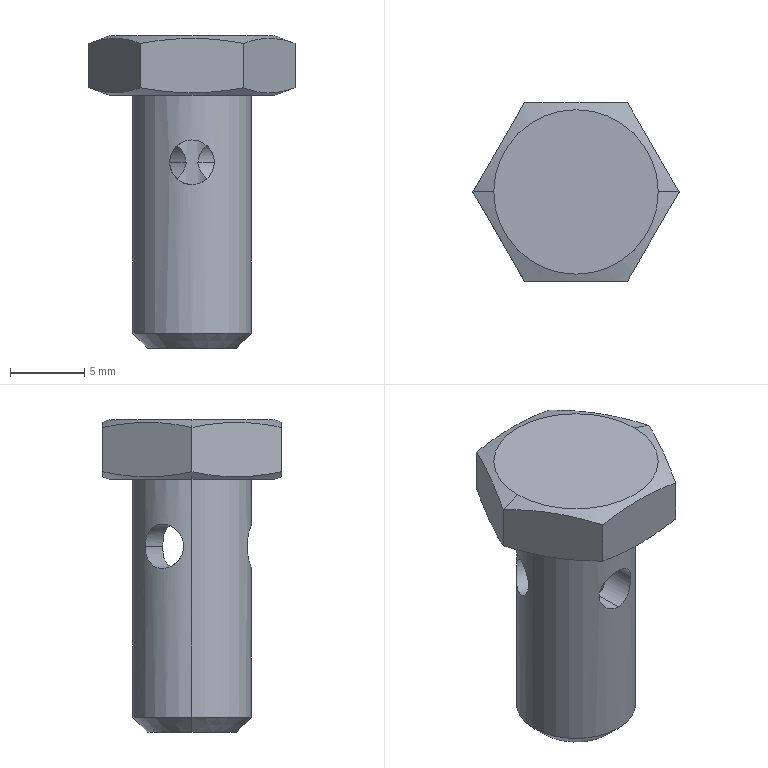Part | SolidWorks | features BaseBody 1 | 1 solid | 26 faces | box 13.856 x 12 x 21 mm | volume 1075 mm3 | cylinder 10 | plane 10 | cone 6 | commonest cylinder face diameters 3 x6 4 x2 8 x2
STEP:
#1=CARTESIAN_POINT('',(-2.461,3.153,-8.5));
#2=VERTEX_POINT('',#1);
#3=CARTESIAN_POINT('',(-3.961,0.555,-8.5));
#4=VERTEX_POINT('',#3);
#5=CARTESIAN_POINT('',(-2.461,3.153,-8.5));
#6=CARTESIAN_POINT('',(-2.461,3.153,-8.4));
#7=CARTESIAN_POINT('',(-2.47,3.147,-8.302));
#8=CARTESIAN_POINT('',(-2.502,3.121,-8.109));
#9=CARTESIAN_POINT('',(-2.527,3.101,-8.013));
#10=CARTESIAN_POINT('',(-2.62,3.024,-7.742));
#11=CARTESIAN_POINT('',(-2.709,2.947,-7.577));
#12=CARTESIAN_POINT('',(-2.911,2.747,-7.303));
#13=CARTESIAN_POINT('',(-3.026,2.623,-7.191));
#14=CARTESIAN_POINT('',(-3.195,2.408,-7.078));
#15=CARTESIAN_POINT('',(-3.252,2.331,-7.049));
#16=CARTESIAN_POINT('',(-3.362,2.17,-7.01));
#17=CARTESIAN_POINT('',(-3.414,2.087,-7.));
#18=CARTESIAN_POINT('',(-3.513,1.916,-7.));
#19=CARTESIAN_POINT('',(-3.56,1.827,-7.01));
#20=CARTESIAN_POINT('',(-3.644,1.653,-7.048));
#21=CARTESIAN_POINT('',(-3.682,1.566,-7.077));
#22=CARTESIAN_POINT('',(-3.784,1.308,-7.191));
#23=CARTESIAN_POINT('',(-3.834,1.148,-7.302));
#24=CARTESIAN_POINT('',(-3.888,0.941,-7.508));
#25=CARTESIAN_POINT('',(-3.903,0.8782,-7.583));
#26=CARTESIAN_POINT('',(-3.926,0.7663,-7.744));
#27=CARTESIAN_POINT('',(-3.935,0.7172,-7.832));
#28=CARTESIAN_POINT('',(-3.956,0.5987,-8.102));
#29=CARTESIAN_POINT('',(-3.961,0.555,-8.3));
#30=CARTESIAN_POINT('',(-3.961,0.555,-8.5));
#31=B_SPLINE_CURVE_WITH_KNOTS('',3,(#5,#6,#7,#8,#9,#10,#11,#12,#13,#14,#15,#16,#17,#18,#19,#20,#21,#22,#23,#24,#25,#26,#27,#28,#29,#30),.UNSPECIFIED.,.F.,.F.,(4,2,2,2,2,2,2,2,2,2,2,2,4),(0.004731,0.005027,0.005322,0.005914,0.006505,0.006801,0.007096,0.007392,0.007688,0.008279,0.008575,0.00887,0.009461),.UNSPECIFIED.);
#32=EDGE_CURVE('',#2,#4,#31,.T.);
#33=ORIENTED_EDGE('',*,*,#32,.T.);
#34=CARTESIAN_POINT('',(-3.961,0.555,-8.5));
#35=CARTESIAN_POINT('',(-3.961,0.555,-8.6));
#36=CARTESIAN_POINT('',(-3.96,0.5656,-8.698));
#37=CARTESIAN_POINT('',(-3.954,0.6067,-8.891));
#38=CARTESIAN_POINT('',(-3.949,0.6378,-8.987));
#39=CARTESIAN_POINT('',(-3.929,0.7568,-9.258));
#40=CARTESIAN_POINT('',(-3.906,0.8722,-9.423));
#41=CARTESIAN_POINT('',(-3.835,1.147,-9.697));
#42=CARTESIAN_POINT('',(-3.784,1.309,-9.809));
#43=CARTESIAN_POINT('',(-3.683,1.563,-9.922));
#44=CARTESIAN_POINT('',(-3.645,1.651,-9.951));
#45=CARTESIAN_POINT('',(-3.56,1.826,-9.99));
#46=CARTESIAN_POINT('',(-3.514,1.913,-10.));
#47=CARTESIAN_POINT('',(-3.416,2.084,-10.));
#48=CARTESIAN_POINT('',(-3.362,2.169,-9.99));
#49=CARTESIAN_POINT('',(-3.253,2.329,-9.952));
#50=CARTESIAN_POINT('',(-3.197,2.406,-9.923));
#51=CARTESIAN_POINT('',(-3.025,2.623,-9.809));
#52=CARTESIAN_POINT('',(-2.911,2.747,-9.698));
#53=CARTESIAN_POINT('',(-2.759,2.897,-9.492));
#54=CARTESIAN_POINT('',(-2.712,2.941,-9.417));
#55=CARTESIAN_POINT('',(-2.627,3.017,-9.256));
#56=CARTESIAN_POINT('',(-2.589,3.05,-9.168));
#57=CARTESIAN_POINT('',(-2.496,3.126,-8.898));
#58=CARTESIAN_POINT('',(-2.461,3.153,-8.7));
#59=CARTESIAN_POINT('',(-2.461,3.153,-8.5));
#60=B_SPLINE_CURVE_WITH_KNOTS('',3,(#34,#35,#36,#37,#38,#39,#40,#41,#42,#43,#44,#45,#46,#47,#48,#49,#50,#51,#52,#53,#54,#55,#56,#57,#58,#59),.UNSPECIFIED.,.F.,.F.,(4,2,2,2,2,2,2,2,2,2,2,2,4),(0.,0.0002957,0.0005914,0.001183,0.001774,0.00207,0.002366,0.002661,0.002957,0.003548,0.003844,0.00414,0.004731),.UNSPECIFIED.);
#61=EDGE_CURVE('',#4,#2,#60,.T.);
#62=ORIENTED_EDGE('',*,*,#61,.T.);
#63=EDGE_LOOP('',(#33,#62));
#64=FACE_BOUND('',#63,.T.);
#65=CARTESIAN_POINT('',(3.961,0.555,-8.5));
#66=VERTEX_POINT('',#65);
#67=CARTESIAN_POINT('',(2.461,3.153,-8.5));
#68=VERTEX_POINT('',#67);
#69=CARTESIAN_POINT('',(3.961,0.555,-8.5));
#70=CARTESIAN_POINT('',(3.961,0.555,-8.4));
#71=CARTESIAN_POINT('',(3.96,0.5656,-8.302));
#72=CARTESIAN_POINT('',(3.954,0.6067,-8.109));
#73=CARTESIAN_POINT('',(3.949,0.6378,-8.013));
#74=CARTESIAN_POINT('',(3.929,0.7568,-7.742));
#75=CARTESIAN_POINT('',(3.906,0.8722,-7.577));
#76=CARTESIAN_POINT('',(3.835,1.147,-7.303));
#77=CARTESIAN_POINT('',(3.784,1.309,-7.191));
#78=CARTESIAN_POINT('',(3.683,1.563,-7.078));
#79=CARTESIAN_POINT('',(3.645,1.651,-7.049));
#80=CARTESIAN_POINT('',(3.56,1.826,-7.01));
#81=CARTESIAN_POINT('',(3.514,1.913,-7.));
#82=CARTESIAN_POINT('',(3.416,2.084,-7.));
#83=CARTESIAN_POINT('',(3.362,2.169,-7.01));
#84=CARTESIAN_POINT('',(3.253,2.329,-7.048));
#85=CARTESIAN_POINT('',(3.197,2.406,-7.077));
#86=CARTESIAN_POINT('',(3.025,2.623,-7.191));
#87=CARTESIAN_POINT('',(2.911,2.747,-7.302));
#88=CARTESIAN_POINT('',(2.759,2.897,-7.508));
#89=CARTESIAN_POINT('',(2.712,2.941,-7.583));
#90=CARTESIAN_POINT('',(2.627,3.017,-7.744));
#91=CARTESIAN_POINT('',(2.589,3.05,-7.832));
#92=CARTESIAN_POINT('',(2.496,3.126,-8.102));
#93=CARTESIAN_POINT('',(2.461,3.153,-8.3));
#94=CARTESIAN_POINT('',(2.461,3.153,-8.5));
#95=B_SPLINE_CURVE_WITH_KNOTS('',3,(#69,#70,#71,#72,#73,#74,#75,#76,#77,#78,#79,#80,#81,#82,#83,#84,#85,#86,#87,#88,#89,#90,#91,#92,#93,#94),.UNSPECIFIED.,.F.,.F.,(4,2,2,2,2,2,2,2,2,2,2,2,4),(0.,0.0002957,0.0005914,0.001183,0.001774,0.00207,0.002366,0.002661,0.002957,0.003548,0.003844,0.00414,0.004731),.UNSPECIFIED.);
#96=EDGE_CURVE('',#66,#68,#95,.T.);
#97=ORIENTED_EDGE('',*,*,#96,.T.);
#98=CARTESIAN_POINT('',(2.461,3.153,-8.5));
#99=CARTESIAN_POINT('',(2.461,3.153,-8.6));
#100=CARTESIAN_POINT('',(2.47,3.147,-8.698));
#101=CARTESIAN_POINT('',(2.502,3.121,-8.891));
#102=CARTESIAN_POINT('',(2.527,3.101,-8.987));
#103=CARTESIAN_POINT('',(2.62,3.024,-9.258));
#104=CARTESIAN_POINT('',(2.709,2.947,-9.423));
#105=CARTESIAN_POINT('',(2.911,2.747,-9.697));
#106=CARTESIAN_POINT('',(3.026,2.623,-9.809));
#107=CARTESIAN_POINT('',(3.195,2.408,-9.922));
#108=CARTESIAN_POINT('',(3.252,2.331,-9.951));
#109=CARTESIAN_POINT('',(3.362,2.17,-9.99));
#110=CARTESIAN_POINT('',(3.414,2.087,-10.));
#111=CARTESIAN_POINT('',(3.513,1.916,-10.));
#112=CARTESIAN_POINT('',(3.56,1.827,-9.99));
#113=CARTESIAN_POINT('',(3.644,1.653,-9.952));
#114=CARTESIAN_POINT('',(3.682,1.566,-9.923));
#115=CARTESIAN_POINT('',(3.784,1.308,-9.809));
#116=CARTESIAN_POINT('',(3.834,1.148,-9.698));
#117=CARTESIAN_POINT('',(3.888,0.941,-9.492));
#118=CARTESIAN_POINT('',(3.903,0.8782,-9.417));
#119=CARTESIAN_POINT('',(3.926,0.7663,-9.256));
#120=CARTESIAN_POINT('',(3.935,0.7172,-9.168));
#121=CARTESIAN_POINT('',(3.956,0.5987,-8.898));
#122=CARTESIAN_POINT('',(3.961,0.555,-8.7));
#123=CARTESIAN_POINT('',(3.961,0.555,-8.5));
#124=B_SPLINE_CURVE_WITH_KNOTS('',3,(#98,#99,#100,#101,#102,#103,#104,#105,#106,#107,#108,#109,#110,#111,#112,#113,#114,#115,#116,#117,#118,#119,#120,#121,#122,#123),.UNSPECIFIED.,.F.,.F.,(4,2,2,2,2,2,2,2,2,2,2,2,4),(0.004731,0.005027,0.005322,0.005914,0.006505,0.006801,0.007096,0.007392,0.007688,0.008279,0.008575,0.00887,0.009461),.UNSPECIFIED.);
#125=EDGE_CURVE('',#68,#66,#124,.T.);
#126=ORIENTED_EDGE('',*,*,#125,.T.);
#127=EDGE_LOOP('',(#97,#126));
#128=FACE_BOUND('',#127,.T.);
#129=CARTESIAN_POINT('',(4.,0.,-20.));
#130=VERTEX_POINT('',#129);
#131=CARTESIAN_POINT('',(-4.,0.,-20.));
#132=VERTEX_POINT('',#131);
#133=CARTESIAN_POINT('',(0.,0.,-20.));
#134=DIRECTION('',(0.,0.,1.));
#135=DIRECTION('',(1.,0.,0.));
#136=AXIS2_PLACEMENT_3D('',#133,#134,#135);
#137=CIRCLE('',#136,4.);
#138=EDGE_CURVE('',#130,#132,#137,.T.);
#139=ORIENTED_EDGE('',*,*,#138,.T.);
#140=CARTESIAN_POINT('',(-4.,0.,-4.));
#141=VERTEX_POINT('',#140);
#142=CARTESIAN_POINT('',(-4.,0.,-20.));
#143=DIRECTION('',(0.,0.,1.));
#144=VECTOR('',#143,1000.);
#145=LINE('',#142,#144);
#146=EDGE_CURVE('',#132,#141,#145,.T.);
#147=ORIENTED_EDGE('',*,*,#146,.T.);
#148=CARTESIAN_POINT('',(4.,0.,-4.));
#149=VERTEX_POINT('',#148);
#150=CARTESIAN_POINT('',(0.,0.,-4.));
#151=DIRECTION('',(0.,0.,-1.));
#152=DIRECTION('',(1.,0.,0.));
#153=AXIS2_PLACEMENT_3D('',#150,#151,#152);
#154=CIRCLE('',#153,4.);
#155=EDGE_CURVE('',#141,#149,#154,.T.);
#156=ORIENTED_EDGE('',*,*,#155,.T.);
#157=CARTESIAN_POINT('',(4.,0.,-20.));
#158=DIRECTION('',(0.,0.,1.));
#159=VECTOR('',#158,1000.);
#160=LINE('',#157,#159);
#161=EDGE_CURVE('',#130,#149,#160,.T.);
#162=ORIENTED_EDGE('',*,*,#161,.F.);
#163=EDGE_LOOP('',(#139,#147,#156,#162));
#164=FACE_OUTER_BOUND('',#163,.T.);
#165=CARTESIAN_POINT('',(0.,0.,-20.));
#166=DIRECTION('',(0.,0.,1.));
#167=DIRECTION('',(1.,0.,0.));
#168=AXIS2_PLACEMENT_3D('',#165,#166,#167);
#169=CYLINDRICAL_SURFACE('',#168,4.);
#170=ADVANCED_FACE('',(#64,#128,#164),#169,.T.);
#171=ORIENTED_EDGE('',*,*,#125,.F.);
#172=CARTESIAN_POINT('',(0.3956,1.96,-8.5));
#173=VERTEX_POINT('',#172);
#174=CARTESIAN_POINT('',(2.731,3.309,-8.5));
#175=DIRECTION('',(-0.866,-0.5,0.));
#176=VECTOR('',#175,1000.);
#177=LINE('',#174,#176);
#178=EDGE_CURVE('',#68,#173,#177,.T.);
#179=ORIENTED_EDGE('',*,*,#178,.T.);
#180=CARTESIAN_POINT('',(2.,0.,-9.618));
#181=VERTEX_POINT('',#180);
#182=CARTESIAN_POINT('',(2.,0.,-9.618));
#183=CARTESIAN_POINT('',(2.,0.1195,-9.711));
#184=CARTESIAN_POINT('',(1.989,0.2466,-9.789));
#185=CARTESIAN_POINT('',(1.937,0.5158,-9.914));
#186=CARTESIAN_POINT('',(1.896,0.6536,-9.958));
#187=CARTESIAN_POINT('',(1.808,0.8575,-9.993));
#188=CARTESIAN_POINT('',(1.774,0.9258,-9.999));
#189=CARTESIAN_POINT('',(1.7,1.056,-10.));
#190=CARTESIAN_POINT('',(1.66,1.118,-9.995));
#191=CARTESIAN_POINT('',(1.528,1.299,-9.964));
#192=CARTESIAN_POINT('',(1.429,1.406,-9.92));
#193=CARTESIAN_POINT('',(1.222,1.589,-9.798));
#194=CARTESIAN_POINT('',(1.116,1.664,-9.721));
#195=CARTESIAN_POINT('',(0.9094,1.785,-9.538));
#196=CARTESIAN_POINT('',(0.8094,1.831,-9.435));
#197=CARTESIAN_POINT('',(0.6281,1.901,-9.203));
#198=CARTESIAN_POINT('',(0.5488,1.924,-9.077));
#199=CARTESIAN_POINT('',(0.4307,1.954,-8.8));
#200=CARTESIAN_POINT('',(0.3956,1.96,-8.652));
#201=CARTESIAN_POINT('',(0.3956,1.96,-8.5));
#202=B_SPLINE_CURVE_WITH_KNOTS('',3,(#182,#183,#184,#185,#186,#187,#188,#189,#190,#191,#192,#193,#194,#195,#196,#197,#198,#199,#200,#201),.UNSPECIFIED.,.F.,.F.,(4,2,2,2,2,2,2,2,2,4),(0.,0.0004483,0.0008965,0.001121,0.001345,0.001793,0.002241,0.00269,0.003138,0.003586),.UNSPECIFIED.);
#203=EDGE_CURVE('',#181,#173,#202,.T.);
#204=ORIENTED_EDGE('',*,*,#203,.F.);
#205=CARTESIAN_POINT('',(1.896,-0.6376,-8.5));
#206=VERTEX_POINT('',#205);
#207=CARTESIAN_POINT('',(1.896,-0.6376,-8.5));
#208=CARTESIAN_POINT('',(1.896,-0.6376,-8.613));
#209=CARTESIAN_POINT('',(1.902,-0.6195,-8.722));
#210=CARTESIAN_POINT('',(1.922,-0.5532,-8.933));
#211=CARTESIAN_POINT('',(1.936,-0.505,-9.034));
#212=CARTESIAN_POINT('',(1.963,-0.3894,-9.223));
#213=CARTESIAN_POINT('',(1.976,-0.3208,-9.311));
#214=CARTESIAN_POINT('',(1.994,-0.1707,-9.474));
#215=CARTESIAN_POINT('',(2.,-0.08869,-9.549));
#216=CARTESIAN_POINT('',(2.,0.,-9.618));
#217=B_SPLINE_CURVE_WITH_KNOTS('',3,(#207,#208,#209,#210,#211,#212,#213,#214,#215,#216),.UNSPECIFIED.,.F.,.F.,(4,2,2,2,4),(-0.00133,-0.0009978,-0.0006652,-0.0003326,0.),.UNSPECIFIED.);
#218=EDGE_CURVE('',#206,#181,#217,.T.);
#219=ORIENTED_EDGE('',*,*,#218,.F.);
#220=CARTESIAN_POINT('',(4.231,0.7106,-8.5));
#221=DIRECTION('',(-0.866,-0.5,0.));
#222=VECTOR('',#221,1000.);
#223=LINE('',#220,#222);
#224=EDGE_CURVE('',#66,#206,#223,.T.);
#225=ORIENTED_EDGE('',*,*,#224,.F.);
#226=EDGE_LOOP('',(#171,#179,#204,#219,#225));
#227=FACE_OUTER_BOUND('',#226,.T.);
#228=CARTESIAN_POINT('',(3.481,2.01,-8.5));
#229=DIRECTION('',(-0.866,-0.5,0.));
#230=DIRECTION('',(0.5,-0.866,0.));
#231=AXIS2_PLACEMENT_3D('',#228,#229,#230);
#232=CYLINDRICAL_SURFACE('',#231,1.5);
#233=ADVANCED_FACE('',(#227),#232,.F.);
#234=CARTESIAN_POINT('',(3.,0.,-21.));
#235=VERTEX_POINT('',#234);
#236=CARTESIAN_POINT('',(-3.,0.,-21.));
#237=VERTEX_POINT('',#236);
#238=CARTESIAN_POINT('',(0.,0.,-21.));
#239=DIRECTION('',(0.,0.,1.));
#240=DIRECTION('',(1.,0.,0.));
#241=AXIS2_PLACEMENT_3D('',#238,#239,#240);
#242=CIRCLE('',#241,3.);
#243=EDGE_CURVE('',#235,#237,#242,.T.);
#244=ORIENTED_EDGE('',*,*,#243,.T.);
#245=CARTESIAN_POINT('',(-4.,0.,-20.));
#246=DIRECTION('',(-0.7071,0.,0.7071));
#247=VECTOR('',#246,1000.);
#248=LINE('',#245,#247);
#249=EDGE_CURVE('',#237,#132,#248,.T.);
#250=ORIENTED_EDGE('',*,*,#249,.T.);
#251=ORIENTED_EDGE('',*,*,#138,.F.);
#252=CARTESIAN_POINT('',(4.,0.,-20.));
#253=DIRECTION('',(0.7071,0.,0.7071));
#254=VECTOR('',#253,1000.);
#255=LINE('',#252,#254);
#256=EDGE_CURVE('',#235,#130,#255,.T.);
#257=ORIENTED_EDGE('',*,*,#256,.F.);
#258=EDGE_LOOP('',(#244,#250,#251,#257));
#259=FACE_OUTER_BOUND('',#258,.T.);
#260=CARTESIAN_POINT('',(0.,0.,-20.));
#261=DIRECTION('',(0.,0.,1.));
#262=DIRECTION('',(1.,0.,0.));
#263=AXIS2_PLACEMENT_3D('',#260,#261,#262);
#264=CONICAL_SURFACE('',#263,4.,0.7854);
#265=ADVANCED_FACE('',(#259),#264,.T.);
#266=CARTESIAN_POINT('',(0.,-4.,-10.));
#267=VERTEX_POINT('',#266);
#268=CARTESIAN_POINT('',(0.,-4.,-7.));
#269=VERTEX_POINT('',#268);
#270=CARTESIAN_POINT('',(0.,-4.,-10.));
#271=CARTESIAN_POINT('',(-0.1001,-4.,-10.));
#272=CARTESIAN_POINT('',(-0.1983,-3.996,-9.99));
#273=CARTESIAN_POINT('',(-0.3912,-3.982,-9.951));
#274=CARTESIAN_POINT('',(-0.4869,-3.971,-9.922));
#275=CARTESIAN_POINT('',(-0.7588,-3.932,-9.809));
#276=CARTESIAN_POINT('',(-0.924,-3.894,-9.697));
#277=CARTESIAN_POINT('',(-1.198,-3.819,-9.423));
#278=CARTESIAN_POINT('',(-1.309,-3.781,-9.258));
#279=CARTESIAN_POINT('',(-1.422,-3.739,-8.988));
#280=CARTESIAN_POINT('',(-1.451,-3.728,-8.893));
#281=CARTESIAN_POINT('',(-1.49,-3.712,-8.699));
#282=CARTESIAN_POINT('',(-1.5,-3.708,-8.601));
#283=CARTESIAN_POINT('',(-1.5,-3.708,-8.403));
#284=CARTESIAN_POINT('',(-1.49,-3.712,-8.303));
#285=CARTESIAN_POINT('',(-1.452,-3.727,-8.109));
#286=CARTESIAN_POINT('',(-1.423,-3.739,-8.015));
#287=CARTESIAN_POINT('',(-1.347,-3.767,-7.833));
#288=CARTESIAN_POINT('',(-1.301,-3.783,-7.747));
#289=CARTESIAN_POINT('',(-1.193,-3.818,-7.585));
#290=CARTESIAN_POINT('',(-1.13,-3.838,-7.509));
#291=CARTESIAN_POINT('',(-0.9926,-3.876,-7.371));
#292=CARTESIAN_POINT('',(-0.9178,-3.894,-7.31));
#293=CARTESIAN_POINT('',(-0.756,-3.929,-7.201));
#294=CARTESIAN_POINT('',(-0.6684,-3.945,-7.154));
#295=CARTESIAN_POINT('',(-0.398,-3.984,-7.041));
#296=CARTESIAN_POINT('',(-0.2001,-4.,-7.));
#297=CARTESIAN_POINT('',(0.,-4.,-7.));
#298=B_SPLINE_CURVE_WITH_KNOTS('',3,(#270,#271,#272,#273,#274,#275,#276,#277,#278,#279,#280,#281,#282,#283,#284,#285,#286,#287,#288,#289,#290,#291,#292,#293,#294,#295,#296,#297),.UNSPECIFIED.,.F.,.F.,(4,2,2,2,2,2,2,2,2,2,2,2,2,4),(0.004731,0.005027,0.005323,0.005914,0.006505,0.006801,0.007097,0.007392,0.007688,0.007983,0.008279,0.008575,0.00887,0.009462),.UNSPECIFIED.);
#299=EDGE_CURVE('',#267,#269,#298,.T.);
#300=ORIENTED_EDGE('',*,*,#299,.F.);
#301=CARTESIAN_POINT('',(0.,-2.,-10.));
#302=VERTEX_POINT('',#301);
#303=CARTESIAN_POINT('',(0.,-4.016,-10.));
#304=DIRECTION('',(0.,1.,0.));
#305=VECTOR('',#304,1000.);
#306=LINE('',#303,#305);
#307=EDGE_CURVE('',#267,#302,#306,.T.);
#308=ORIENTED_EDGE('',*,*,#307,.T.);
#309=CARTESIAN_POINT('',(0.,-2.,-7.));
#310=VERTEX_POINT('',#309);
#311=CARTESIAN_POINT('',(0.,-2.,-7.));
#312=CARTESIAN_POINT('',(-0.104,-2.,-7.));
#313=CARTESIAN_POINT('',(-0.2056,-1.992,-7.011));
#314=CARTESIAN_POINT('',(-0.4042,-1.961,-7.052));
#315=CARTESIAN_POINT('',(-0.5017,-1.938,-7.083));
#316=CARTESIAN_POINT('',(-0.7738,-1.854,-7.2));
#317=CARTESIAN_POINT('',(-0.934,-1.775,-7.311));
#318=CARTESIAN_POINT('',(-1.199,-1.609,-7.579));
#319=CARTESIAN_POINT('',(-1.304,-1.52,-7.735));
#320=CARTESIAN_POINT('',(-1.418,-1.412,-8.001));
#321=CARTESIAN_POINT('',(-1.448,-1.38,-8.096));
#322=CARTESIAN_POINT('',(-1.489,-1.336,-8.292));
#323=CARTESIAN_POINT('',(-1.5,-1.323,-8.396));
#324=CARTESIAN_POINT('',(-1.5,-1.323,-8.601));
#325=CARTESIAN_POINT('',(-1.489,-1.335,-8.705));
#326=CARTESIAN_POINT('',(-1.449,-1.379,-8.902));
#327=CARTESIAN_POINT('',(-1.419,-1.411,-8.997));
#328=CARTESIAN_POINT('',(-1.343,-1.483,-9.175));
#329=CARTESIAN_POINT('',(-1.298,-1.523,-9.258));
#330=CARTESIAN_POINT('',(-1.193,-1.606,-9.414));
#331=CARTESIAN_POINT('',(-1.133,-1.65,-9.487));
#332=CARTESIAN_POINT('',(-1.001,-1.733,-9.621));
#333=CARTESIAN_POINT('',(-0.929,-1.773,-9.682));
#334=CARTESIAN_POINT('',(-0.7712,-1.847,-9.79));
#335=CARTESIAN_POINT('',(-0.6846,-1.882,-9.838));
#336=CARTESIAN_POINT('',(-0.4127,-1.966,-9.956));
#337=CARTESIAN_POINT('',(-0.2078,-2.,-10.));
#338=CARTESIAN_POINT('',(0.,-2.,-10.));
#339=B_SPLINE_CURVE_WITH_KNOTS('',3,(#311,#312,#313,#314,#315,#316,#317,#318,#319,#320,#321,#322,#323,#324,#325,#326,#327,#328,#329,#330,#331,#332,#333,#334,#335,#336,#337,#338),.UNSPECIFIED.,.F.,.F.,(4,2,2,2,2,2,2,2,2,2,2,2,2,4),(0.004911,0.005217,0.005524,0.006137,0.00675,0.007056,0.007363,0.00767,0.007976,0.008283,0.008589,0.008896,0.009202,0.009815),.UNSPECIFIED.);
#340=EDGE_CURVE('',#310,#302,#339,.T.);
#341=ORIENTED_EDGE('',*,*,#340,.F.);
#342=CARTESIAN_POINT('',(0.,-4.016,-7.));
#343=DIRECTION('',(0.,1.,0.));
#344=VECTOR('',#343,1000.);
#345=LINE('',#342,#344);
#346=EDGE_CURVE('',#269,#310,#345,.T.);
#347=ORIENTED_EDGE('',*,*,#346,.F.);
#348=EDGE_LOOP('',(#300,#308,#341,#347));
#349=FACE_OUTER_BOUND('',#348,.T.);
#350=CARTESIAN_POINT('',(0.,-4.016,-8.5));
#351=DIRECTION('',(0.,1.,0.));
#352=DIRECTION('',(0.,0.,1.));
#353=AXIS2_PLACEMENT_3D('',#350,#351,#352);
#354=CYLINDRICAL_SURFACE('',#353,1.5);
#355=ADVANCED_FACE('',(#349),#354,.F.);
#356=ORIENTED_EDGE('',*,*,#340,.T.);
#357=CARTESIAN_POINT('',(0.,-2.,-10.));
#358=CARTESIAN_POINT('',(0.104,-2.,-10.));
#359=CARTESIAN_POINT('',(0.2056,-1.992,-9.989));
#360=CARTESIAN_POINT('',(0.4042,-1.961,-9.948));
#361=CARTESIAN_POINT('',(0.5017,-1.938,-9.917));
#362=CARTESIAN_POINT('',(0.7738,-1.854,-9.8));
#363=CARTESIAN_POINT('',(0.934,-1.775,-9.689));
#364=CARTESIAN_POINT('',(1.199,-1.609,-9.421));
#365=CARTESIAN_POINT('',(1.304,-1.52,-9.265));
#366=CARTESIAN_POINT('',(1.418,-1.412,-8.999));
#367=CARTESIAN_POINT('',(1.448,-1.38,-8.904));
#368=CARTESIAN_POINT('',(1.489,-1.336,-8.708));
#369=CARTESIAN_POINT('',(1.5,-1.323,-8.604));
#370=CARTESIAN_POINT('',(1.5,-1.323,-8.399));
#371=CARTESIAN_POINT('',(1.489,-1.335,-8.295));
#372=CARTESIAN_POINT('',(1.449,-1.379,-8.098));
#373=CARTESIAN_POINT('',(1.419,-1.411,-8.003));
#374=CARTESIAN_POINT('',(1.343,-1.483,-7.825));
#375=CARTESIAN_POINT('',(1.298,-1.523,-7.742));
#376=CARTESIAN_POINT('',(1.193,-1.606,-7.586));
#377=CARTESIAN_POINT('',(1.133,-1.65,-7.513));
#378=CARTESIAN_POINT('',(1.001,-1.733,-7.379));
#379=CARTESIAN_POINT('',(0.929,-1.773,-7.318));
#380=CARTESIAN_POINT('',(0.7712,-1.847,-7.21));
#381=CARTESIAN_POINT('',(0.6846,-1.882,-7.162));
#382=CARTESIAN_POINT('',(0.4127,-1.966,-7.044));
#383=CARTESIAN_POINT('',(0.2082,-2.,-7.));
#384=CARTESIAN_POINT('',(0.,-2.,-7.));
#385=B_SPLINE_CURVE_WITH_KNOTS('',3,(#357,#358,#359,#360,#361,#362,#363,#364,#365,#366,#367,#368,#369,#370,#371,#372,#373,#374,#375,#376,#377,#378,#379,#380,#381,#382,#383,#384),.UNSPECIFIED.,.F.,.F.,(4,2,2,2,2,2,2,2,2,2,2,2,2,4),(0.,0.0003069,0.0006138,0.001228,0.001841,0.002148,0.002455,0.002762,0.003069,0.003376,0.003683,0.00399,0.004297,0.004911),.UNSPECIFIED.);
#386=EDGE_CURVE('',#302,#310,#385,.T.);
#387=ORIENTED_EDGE('',*,*,#386,.T.);
#388=EDGE_LOOP('',(#356,#387));
#389=FACE_BOUND('',#388,.T.);
#390=CARTESIAN_POINT('',(-2.,0.,-21.));
#391=VERTEX_POINT('',#390);
#392=CARTESIAN_POINT('',(2.,0.,-21.));
#393=VERTEX_POINT('',#392);
#394=CARTESIAN_POINT('',(0.,0.,-21.));
#395=DIRECTION('',(0.,0.,1.));
#396=DIRECTION('',(1.,0.,0.));
#397=AXIS2_PLACEMENT_3D('',#394,#395,#396);
#398=CIRCLE('',#397,2.);
#399=EDGE_CURVE('',#391,#393,#398,.T.);
#400=ORIENTED_EDGE('',*,*,#399,.F.);
#401=CARTESIAN_POINT('',(-2.,0.,-9.618));
#402=VERTEX_POINT('',#401);
#403=CARTESIAN_POINT('',(-2.,0.,-21.));
#404=DIRECTION('',(0.,0.,1.));
#405=VECTOR('',#404,1000.);
#406=LINE('',#403,#405);
#407=EDGE_CURVE('',#391,#402,#406,.T.);
#408=ORIENTED_EDGE('',*,*,#407,.T.);
#409=CARTESIAN_POINT('',(-1.896,-0.6376,-8.5));
#410=VERTEX_POINT('',#409);
#411=CARTESIAN_POINT('',(-1.896,-0.6376,-8.5));
#412=CARTESIAN_POINT('',(-1.896,-0.6376,-8.613));
#413=CARTESIAN_POINT('',(-1.902,-0.6196,-8.721));
#414=CARTESIAN_POINT('',(-1.922,-0.5535,-8.932));
#415=CARTESIAN_POINT('',(-1.936,-0.5054,-9.034));
#416=CARTESIAN_POINT('',(-1.976,-0.3324,-9.316));
#417=CARTESIAN_POINT('',(-2.,-0.177,-9.481));
#418=CARTESIAN_POINT('',(-2.,0.,-9.618));
#419=B_SPLINE_CURVE_WITH_KNOTS('',3,(#411,#412,#413,#414,#415,#416,#417,#418),.UNSPECIFIED.,.F.,.F.,(4,2,2,4),(0.004899,0.005229,0.00556,0.006221),.UNSPECIFIED.);
#420=EDGE_CURVE('',#410,#402,#419,.T.);
#421=ORIENTED_EDGE('',*,*,#420,.F.);
#422=CARTESIAN_POINT('',(-2.,0.,-7.382));
#423=VERTEX_POINT('',#422);
#424=CARTESIAN_POINT('',(-2.,0.,-7.382));
#425=CARTESIAN_POINT('',(-2.,-0.08867,-7.451));
#426=CARTESIAN_POINT('',(-1.994,-0.1705,-7.525));
#427=CARTESIAN_POINT('',(-1.976,-0.32,-7.688));
#428=CARTESIAN_POINT('',(-1.963,-0.3885,-7.776));
#429=CARTESIAN_POINT('',(-1.923,-0.5625,-8.059));
#430=CARTESIAN_POINT('',(-1.896,-0.6376,-8.275));
#431=CARTESIAN_POINT('',(-1.896,-0.6376,-8.5));
#432=B_SPLINE_CURVE_WITH_KNOTS('',3,(#424,#425,#426,#427,#428,#429,#430,#431),.UNSPECIFIED.,.F.,.F.,(4,2,2,4),(0.003576,0.003907,0.004238,0.004899),.UNSPECIFIED.);
#433=EDGE_CURVE('',#423,#410,#432,.T.);
#434=ORIENTED_EDGE('',*,*,#433,.F.);
#435=CARTESIAN_POINT('',(-2.,0.,-4.));
#436=VERTEX_POINT('',#435);
#437=CARTESIAN_POINT('',(-2.,0.,-21.));
#438=DIRECTION('',(0.,0.,1.));
#439=VECTOR('',#438,1000.);
#440=LINE('',#437,#439);
#441=EDGE_CURVE('',#423,#436,#440,.T.);
#442=ORIENTED_EDGE('',*,*,#441,.T.);
#443=CARTESIAN_POINT('',(2.,0.,-4.));
#444=VERTEX_POINT('',#443);
#445=CARTESIAN_POINT('',(0.,0.,-4.));
#446=DIRECTION('',(0.,0.,-1.));
#447=DIRECTION('',(1.,0.,0.));
#448=AXIS2_PLACEMENT_3D('',#445,#446,#447);
#449=CIRCLE('',#448,2.);
#450=EDGE_CURVE('',#444,#436,#449,.T.);
#451=ORIENTED_EDGE('',*,*,#450,.F.);
#452=CARTESIAN_POINT('',(2.,0.,-7.382));
#453=VERTEX_POINT('',#452);
#454=CARTESIAN_POINT('',(2.,0.,-21.));
#455=DIRECTION('',(0.,0.,1.));
#456=VECTOR('',#455,1000.);
#457=LINE('',#454,#456);
#458=EDGE_CURVE('',#453,#444,#457,.T.);
#459=ORIENTED_EDGE('',*,*,#458,.F.);
#460=CARTESIAN_POINT('',(2.,0.,-7.382));
#461=CARTESIAN_POINT('',(2.,-0.1769,-7.519));
#462=CARTESIAN_POINT('',(1.976,-0.3312,-7.683));
#463=CARTESIAN_POINT('',(1.923,-0.562,-8.058));
#464=CARTESIAN_POINT('',(1.896,-0.6376,-8.275));
#465=CARTESIAN_POINT('',(1.896,-0.6376,-8.5));
#466=B_SPLINE_CURVE_WITH_KNOTS('',3,(#460,#461,#462,#463,#464,#465),.UNSPECIFIED.,.F.,.F.,(4,2,4),(0.007178,0.00784,0.008503),.UNSPECIFIED.);
#467=EDGE_CURVE('',#453,#206,#466,.T.);
#468=ORIENTED_EDGE('',*,*,#467,.T.);
#469=ORIENTED_EDGE('',*,*,#218,.T.);
#470=CARTESIAN_POINT('',(2.,0.,-21.));
#471=DIRECTION('',(0.,0.,1.));
#472=VECTOR('',#471,1000.);
#473=LINE('',#470,#472);
#474=EDGE_CURVE('',#393,#181,#473,.T.);
#475=ORIENTED_EDGE('',*,*,#474,.F.);
#476=EDGE_LOOP('',(#400,#408,#421,#434,#442,#451,#459,#468,#469,#475));
#477=FACE_OUTER_BOUND('',#476,.T.);
#478=CARTESIAN_POINT('',(0.,0.,-21.));
#479=DIRECTION('',(0.,0.,1.));
#480=DIRECTION('',(1.,0.,0.));
#481=AXIS2_PLACEMENT_3D('',#478,#479,#480);
#482=CYLINDRICAL_SURFACE('',#481,2.);
#483=ADVANCED_FACE('',(#389,#477),#482,.F.);
#484=ORIENTED_EDGE('',*,*,#61,.F.);
#485=CARTESIAN_POINT('',(-4.231,0.7106,-8.5));
#486=DIRECTION('',(0.866,-0.5,0.));
#487=VECTOR('',#486,1000.);
#488=LINE('',#485,#487);
#489=EDGE_CURVE('',#4,#410,#488,.T.);
#490=ORIENTED_EDGE('',*,*,#489,.T.);
#491=ORIENTED_EDGE('',*,*,#420,.T.);
#492=CARTESIAN_POINT('',(-0.3956,1.96,-8.5));
#493=VERTEX_POINT('',#492);
#494=CARTESIAN_POINT('',(-2.,0.,-9.618));
#495=CARTESIAN_POINT('',(-2.,0.1195,-9.711));
#496=CARTESIAN_POINT('',(-1.989,0.2466,-9.789));
#497=CARTESIAN_POINT('',(-1.937,0.5158,-9.914));
#498=CARTESIAN_POINT('',(-1.896,0.6536,-9.958));
#499=CARTESIAN_POINT('',(-1.808,0.8575,-9.993));
#500=CARTESIAN_POINT('',(-1.774,0.9258,-9.999));
#501=CARTESIAN_POINT('',(-1.7,1.056,-10.));
#502=CARTESIAN_POINT('',(-1.66,1.118,-9.995));
#503=CARTESIAN_POINT('',(-1.528,1.298,-9.964));
#504=CARTESIAN_POINT('',(-1.429,1.406,-9.92));
#505=CARTESIAN_POINT('',(-1.222,1.589,-9.798));
#506=CARTESIAN_POINT('',(-1.116,1.664,-9.721));
#507=CARTESIAN_POINT('',(-0.9094,1.785,-9.538));
#508=CARTESIAN_POINT('',(-0.8094,1.831,-9.435));
#509=CARTESIAN_POINT('',(-0.6281,1.901,-9.203));
#510=CARTESIAN_POINT('',(-0.5488,1.924,-9.077));
#511=CARTESIAN_POINT('',(-0.4307,1.954,-8.8));
#512=CARTESIAN_POINT('',(-0.3956,1.96,-8.652));
#513=CARTESIAN_POINT('',(-0.3956,1.96,-8.5));
#514=B_SPLINE_CURVE_WITH_KNOTS('',3,(#494,#495,#496,#497,#498,#499,#500,#501,#502,#503,#504,#505,#506,#507,#508,#509,#510,#511,#512,#513),.UNSPECIFIED.,.F.,.F.,(4,2,2,2,2,2,2,2,2,4),(-0.003571,-0.003124,-0.002678,-0.002455,-0.002232,-0.001785,-0.001339,-0.0008927,-0.0004463,0.),.UNSPECIFIED.);
#515=EDGE_CURVE('',#402,#493,#514,.T.);
#516=ORIENTED_EDGE('',*,*,#515,.T.);
#517=CARTESIAN_POINT('',(-2.731,3.309,-8.5));
#518=DIRECTION('',(0.866,-0.5,0.));
#519=VECTOR('',#518,1000.);
#520=LINE('',#517,#519);
#521=EDGE_CURVE('',#2,#493,#520,.T.);
#522=ORIENTED_EDGE('',*,*,#521,.F.);
#523=EDGE_LOOP('',(#484,#490,#491,#516,#522));
#524=FACE_OUTER_BOUND('',#523,.T.);
#525=CARTESIAN_POINT('',(-3.481,2.01,-8.5));
#526=DIRECTION('',(0.866,-0.5,0.));
#527=DIRECTION('',(0.5,0.866,0.));
#528=AXIS2_PLACEMENT_3D('',#525,#526,#527);
#529=CYLINDRICAL_SURFACE('',#528,1.5);
#530=ADVANCED_FACE('',(#524),#529,.F.);
#531=CARTESIAN_POINT('',(5.528,0.,-4.));
#532=VERTEX_POINT('',#531);
#533=CARTESIAN_POINT('',(-5.528,0.,-4.));
#534=VERTEX_POINT('',#533);
#535=CARTESIAN_POINT('',(0.,0.,-4.));
#536=DIRECTION('',(0.,0.,1.));
#537=DIRECTION('',(1.,0.,0.));
#538=AXIS2_PLACEMENT_3D('',#535,#536,#537);
#539=CIRCLE('',#538,5.528);
#540=EDGE_CURVE('',#532,#534,#539,.T.);
#541=ORIENTED_EDGE('',*,*,#540,.T.);
#542=CARTESIAN_POINT('',(-6.928,0.000000026,-3.49));
#543=VERTEX_POINT('',#542);
#544=CARTESIAN_POINT('',(-6.937,0.,-3.487));
#545=DIRECTION('',(-0.9397,0.,0.342));
#546=VECTOR('',#545,1000.);
#547=LINE('',#544,#546);
#548=EDGE_CURVE('',#534,#543,#547,.T.);
#549=ORIENTED_EDGE('',*,*,#548,.T.);
#550=CARTESIAN_POINT('',(-3.464,6.,-3.49));
#551=VERTEX_POINT('',#550);
#552=CARTESIAN_POINT('',(-6.928,0.000000026,-3.49));
#553=CARTESIAN_POINT('',(-6.351,1.,-3.701));
#554=CARTESIAN_POINT('',(-5.196,3.,-3.956));
#555=CARTESIAN_POINT('',(-4.041,5.,-3.701));
#556=CARTESIAN_POINT('',(-3.464,6.,-3.49));
#557=B_SPLINE_CURVE_WITH_KNOTS('',3,(#552,#553,#554,#555,#556),.UNSPECIFIED.,.F.,.F.,(4,1,4),(0.,0.003464,0.006928),.UNSPECIFIED.);
#558=EDGE_CURVE('',#543,#551,#557,.T.);
#559=ORIENTED_EDGE('',*,*,#558,.T.);
#560=CARTESIAN_POINT('',(3.464,6.,-3.49));
#561=VERTEX_POINT('',#560);
#562=CARTESIAN_POINT('',(-3.464,6.,-3.49));
#563=CARTESIAN_POINT('',(-2.309,6.,-3.701));
#564=CARTESIAN_POINT('',(-0.000000061,6.,-3.956));
#565=CARTESIAN_POINT('',(2.309,6.,-3.701));
#566=CARTESIAN_POINT('',(3.464,6.,-3.49));
#567=B_SPLINE_CURVE_WITH_KNOTS('',3,(#562,#563,#564,#565,#566),.UNSPECIFIED.,.F.,.F.,(4,1,4),(0.,0.003464,0.006928),.UNSPECIFIED.);
#568=EDGE_CURVE('',#551,#561,#567,.T.);
#569=ORIENTED_EDGE('',*,*,#568,.T.);
#570=CARTESIAN_POINT('',(6.928,-0.000000001,-3.49));
#571=VERTEX_POINT('',#570);
#572=CARTESIAN_POINT('',(3.464,6.,-3.49));
#573=CARTESIAN_POINT('',(4.041,5.,-3.701));
#574=CARTESIAN_POINT('',(5.196,3.,-3.956));
#575=CARTESIAN_POINT('',(6.351,1.,-3.701));
#576=CARTESIAN_POINT('',(6.928,-0.000000001,-3.49));
#577=B_SPLINE_CURVE_WITH_KNOTS('',3,(#572,#573,#574,#575,#576),.UNSPECIFIED.,.F.,.F.,(4,1,4),(0.,0.003464,0.006928),.UNSPECIFIED.);
#578=EDGE_CURVE('',#561,#571,#577,.T.);
#579=ORIENTED_EDGE('',*,*,#578,.T.);
#580=CARTESIAN_POINT('',(6.937,0.,-3.487));
#581=DIRECTION('',(0.9397,0.,0.342));
#582=VECTOR('',#581,1000.);
#583=LINE('',#580,#582);
#584=EDGE_CURVE('',#532,#571,#583,.T.);
#585=ORIENTED_EDGE('',*,*,#584,.F.);
#586=EDGE_LOOP('',(#541,#549,#559,#569,#579,#585));
#587=FACE_OUTER_BOUND('',#586,.T.);
#588=CARTESIAN_POINT('',(0.,0.,-3.487));
#589=DIRECTION('',(0.,0.,1.));
#590=DIRECTION('',(1.,0.,0.));
#591=AXIS2_PLACEMENT_3D('',#588,#589,#590);
#592=CONICAL_SURFACE('',#591,6.937,1.222);
#593=ADVANCED_FACE('',(#587),#592,.T.);
#594=CARTESIAN_POINT('',(-5.528,0.,0.));
#595=VERTEX_POINT('',#594);
#596=CARTESIAN_POINT('',(5.528,0.,0.));
#597=VERTEX_POINT('',#596);
#598=CARTESIAN_POINT('',(0.,0.,0.));
#599=DIRECTION('',(0.,0.,-1.));
#600=DIRECTION('',(-1.,0.,0.));
#601=AXIS2_PLACEMENT_3D('',#598,#599,#600);
#602=CIRCLE('',#601,5.528);
#603=EDGE_CURVE('',#595,#597,#602,.T.);
#604=ORIENTED_EDGE('',*,*,#603,.T.);
#605=CARTESIAN_POINT('',(6.928,-0.000000001,-0.5096));
#606=VERTEX_POINT('',#605);
#607=CARTESIAN_POINT('',(6.937,0.,-0.5126));
#608=DIRECTION('',(0.9397,0.,-0.342));
#609=VECTOR('',#608,1000.);
#610=LINE('',#607,#609);
#611=EDGE_CURVE('',#597,#606,#610,.T.);
#612=ORIENTED_EDGE('',*,*,#611,.T.);
#613=CARTESIAN_POINT('',(3.464,6.,-0.5096));
#614=VERTEX_POINT('',#613);
#615=CARTESIAN_POINT('',(3.464,6.,-0.5096));
#616=CARTESIAN_POINT('',(4.041,5.,-0.2994));
#617=CARTESIAN_POINT('',(5.196,3.,-0.04402));
#618=CARTESIAN_POINT('',(6.351,1.,-0.2994));
#619=CARTESIAN_POINT('',(6.928,-0.000000001,-0.5096));
#620=B_SPLINE_CURVE_WITH_KNOTS('',3,(#615,#616,#617,#618,#619),.UNSPECIFIED.,.F.,.F.,(4,1,4),(0.,0.003464,0.006928),.UNSPECIFIED.);
#621=EDGE_CURVE('',#614,#606,#620,.T.);
#622=ORIENTED_EDGE('',*,*,#621,.F.);
#623=CARTESIAN_POINT('',(-3.464,6.,-0.5096));
#624=VERTEX_POINT('',#623);
#625=CARTESIAN_POINT('',(-3.464,6.,-0.5096));
#626=CARTESIAN_POINT('',(-2.309,6.,-0.2994));
#627=CARTESIAN_POINT('',(0.,6.,-0.04402));
#628=CARTESIAN_POINT('',(2.309,6.,-0.2994));
#629=CARTESIAN_POINT('',(3.464,6.,-0.5096));
#630=B_SPLINE_CURVE_WITH_KNOTS('',3,(#625,#626,#627,#628,#629),.UNSPECIFIED.,.F.,.F.,(4,1,4),(0.,0.003464,0.006928),.UNSPECIFIED.);
#631=EDGE_CURVE('',#624,#614,#630,.T.);
#632=ORIENTED_EDGE('',*,*,#631,.F.);
#633=CARTESIAN_POINT('',(-6.928,0.,-0.5096));
#634=VERTEX_POINT('',#633);
#635=CARTESIAN_POINT('',(-3.464,6.,-0.5096));
#636=CARTESIAN_POINT('',(-4.041,5.,-0.2994));
#637=CARTESIAN_POINT('',(-5.196,3.,-0.04402));
#638=CARTESIAN_POINT('',(-6.351,1.,-0.2994));
#639=CARTESIAN_POINT('',(-6.928,0.,-0.5096));
#640=B_SPLINE_CURVE_WITH_KNOTS('',3,(#635,#636,#637,#638,#639),.UNSPECIFIED.,.F.,.F.,(4,1,4),(0.,0.003464,0.006928),.UNSPECIFIED.);
#641=EDGE_CURVE('',#624,#634,#640,.T.);
#642=ORIENTED_EDGE('',*,*,#641,.T.);
#643=CARTESIAN_POINT('',(-6.937,0.,-0.5126));
#644=DIRECTION('',(-0.9397,0.,-0.342));
#645=VECTOR('',#644,1000.);
#646=LINE('',#643,#645);
#647=EDGE_CURVE('',#595,#634,#646,.T.);
#648=ORIENTED_EDGE('',*,*,#647,.F.);
#649=EDGE_LOOP('',(#604,#612,#622,#632,#642,#648));
#650=FACE_OUTER_BOUND('',#649,.T.);
#651=CARTESIAN_POINT('',(0.,0.,-0.5126));
#652=DIRECTION('',(0.,0.,-1.));
#653=DIRECTION('',(-1.,0.,0.));
#654=AXIS2_PLACEMENT_3D('',#651,#652,#653);
#655=CONICAL_SURFACE('',#654,6.937,1.222);
#656=ADVANCED_FACE('',(#650),#655,.T.);
#657=ORIENTED_EDGE('',*,*,#146,.F.);
#658=CARTESIAN_POINT('',(0.,0.,-20.));
#659=DIRECTION('',(0.,0.,1.));
#660=DIRECTION('',(1.,0.,0.));
#661=AXIS2_PLACEMENT_3D('',#658,#659,#660);
#662=CIRCLE('',#661,4.);
#663=EDGE_CURVE('',#132,#130,#662,.T.);
#664=ORIENTED_EDGE('',*,*,#663,.T.);
#665=ORIENTED_EDGE('',*,*,#161,.T.);
#666=CARTESIAN_POINT('',(0.,0.,-4.));
#667=DIRECTION('',(0.,0.,-1.));
#668=DIRECTION('',(1.,0.,0.));
#669=AXIS2_PLACEMENT_3D('',#666,#667,#668);
#670=CIRCLE('',#669,4.);
#671=EDGE_CURVE('',#149,#141,#670,.T.);
#672=ORIENTED_EDGE('',*,*,#671,.T.);
#673=EDGE_LOOP('',(#657,#664,#665,#672));
#674=FACE_OUTER_BOUND('',#673,.T.);
#675=CARTESIAN_POINT('',(0.,-4.,-7.));
#676=CARTESIAN_POINT('',(0.1001,-4.,-7.));
#677=CARTESIAN_POINT('',(0.1983,-3.996,-7.01));
#678=CARTESIAN_POINT('',(0.3912,-3.982,-7.049));
#679=CARTESIAN_POINT('',(0.4869,-3.971,-7.078));
#680=CARTESIAN_POINT('',(0.7588,-3.932,-7.191));
#681=CARTESIAN_POINT('',(0.924,-3.894,-7.303));
#682=CARTESIAN_POINT('',(1.198,-3.819,-7.577));
#683=CARTESIAN_POINT('',(1.309,-3.781,-7.742));
#684=CARTESIAN_POINT('',(1.422,-3.739,-8.012));
#685=CARTESIAN_POINT('',(1.451,-3.728,-8.107));
#686=CARTESIAN_POINT('',(1.49,-3.712,-8.301));
#687=CARTESIAN_POINT('',(1.5,-3.708,-8.399));
#688=CARTESIAN_POINT('',(1.5,-3.708,-8.597));
#689=CARTESIAN_POINT('',(1.49,-3.712,-8.697));
#690=CARTESIAN_POINT('',(1.452,-3.727,-8.891));
#691=CARTESIAN_POINT('',(1.423,-3.739,-8.985));
#692=CARTESIAN_POINT('',(1.347,-3.767,-9.167));
#693=CARTESIAN_POINT('',(1.301,-3.783,-9.253));
#694=CARTESIAN_POINT('',(1.193,-3.818,-9.415));
#695=CARTESIAN_POINT('',(1.13,-3.838,-9.491));
#696=CARTESIAN_POINT('',(0.9926,-3.876,-9.629));
#697=CARTESIAN_POINT('',(0.9178,-3.894,-9.69));
#698=CARTESIAN_POINT('',(0.756,-3.929,-9.799));
#699=CARTESIAN_POINT('',(0.6684,-3.945,-9.846));
#700=CARTESIAN_POINT('',(0.398,-3.984,-9.959));
#701=CARTESIAN_POINT('',(0.2002,-4.,-10.));
#702=CARTESIAN_POINT('',(0.,-4.,-10.));
#703=B_SPLINE_CURVE_WITH_KNOTS('',3,(#675,#676,#677,#678,#679,#680,#681,#682,#683,#684,#685,#686,#687,#688,#689,#690,#691,#692,#693,#694,#695,#696,#697,#698,#699,#700,#701,#702),.UNSPECIFIED.,.F.,.F.,(4,2,2,2,2,2,2,2,2,2,2,2,2,4),(0.,0.0002957,0.0005914,0.001183,0.001774,0.00207,0.002366,0.002661,0.002957,0.003253,0.003549,0.003844,0.00414,0.004731),.UNSPECIFIED.);
#704=EDGE_CURVE('',#269,#267,#703,.T.);
#705=ORIENTED_EDGE('',*,*,#704,.T.);
#706=ORIENTED_EDGE('',*,*,#299,.T.);
#707=EDGE_LOOP('',(#705,#706));
#708=FACE_BOUND('',#707,.T.);
#709=CARTESIAN_POINT('',(0.,0.,-20.));
#710=DIRECTION('',(0.,0.,1.));
#711=DIRECTION('',(1.,0.,0.));
#712=AXIS2_PLACEMENT_3D('',#709,#710,#711);
#713=CYLINDRICAL_SURFACE('',#712,4.);
#714=ADVANCED_FACE('',(#674,#708),#713,.T.);
#715=ORIENTED_EDGE('',*,*,#178,.F.);
#716=ORIENTED_EDGE('',*,*,#96,.F.);
#717=ORIENTED_EDGE('',*,*,#224,.T.);
#718=ORIENTED_EDGE('',*,*,#467,.F.);
#719=CARTESIAN_POINT('',(0.3956,1.96,-8.5));
#720=CARTESIAN_POINT('',(0.3956,1.96,-8.348));
#721=CARTESIAN_POINT('',(0.4301,1.954,-8.202));
#722=CARTESIAN_POINT('',(0.5477,1.925,-7.925));
#723=CARTESIAN_POINT('',(0.6268,1.902,-7.799));
#724=CARTESIAN_POINT('',(0.8079,1.832,-7.567));
#725=CARTESIAN_POINT('',(0.9067,1.787,-7.464));
#726=CARTESIAN_POINT('',(1.112,1.666,-7.282));
#727=CARTESIAN_POINT('',(1.219,1.591,-7.204));
#728=CARTESIAN_POINT('',(1.425,1.41,-7.082));
#729=CARTESIAN_POINT('',(1.525,1.303,-7.038));
#730=CARTESIAN_POINT('',(1.699,1.065,-6.994));
#731=CARTESIAN_POINT('',(1.776,0.931,-6.995));
#732=CARTESIAN_POINT('',(1.894,0.6594,-7.04));
#733=CARTESIAN_POINT('',(1.936,0.5186,-7.085));
#734=CARTESIAN_POINT('',(1.989,0.25,-7.21));
#735=CARTESIAN_POINT('',(2.,0.1199,-7.289));
#736=CARTESIAN_POINT('',(2.,0.,-7.382));
#737=B_SPLINE_CURVE_WITH_KNOTS('',3,(#719,#720,#721,#722,#723,#724,#725,#726,#727,#728,#729,#730,#731,#732,#733,#734,#735,#736),.UNSPECIFIED.,.F.,.F.,(4,2,2,2,2,2,2,2,4),(0.003586,0.004035,0.004484,0.004933,0.005382,0.005831,0.00628,0.006729,0.007178),.UNSPECIFIED.);
#738=EDGE_CURVE('',#173,#453,#737,.T.);
#739=ORIENTED_EDGE('',*,*,#738,.F.);
#740=EDGE_LOOP('',(#715,#716,#717,#718,#739));
#741=FACE_OUTER_BOUND('',#740,.T.);
#742=CARTESIAN_POINT('',(3.481,2.01,-8.5));
#743=DIRECTION('',(-0.866,-0.5,0.));
#744=DIRECTION('',(0.5,-0.866,0.));
#745=AXIS2_PLACEMENT_3D('',#742,#743,#744);
#746=CYLINDRICAL_SURFACE('',#745,1.5);
#747=ADVANCED_FACE('',(#741),#746,.F.);
#748=ORIENTED_EDGE('',*,*,#249,.F.);
#749=CARTESIAN_POINT('',(0.,0.,-21.));
#750=DIRECTION('',(0.,0.,1.));
#751=DIRECTION('',(1.,0.,0.));
#752=AXIS2_PLACEMENT_3D('',#749,#750,#751);
#753=CIRCLE('',#752,3.);
#754=EDGE_CURVE('',#237,#235,#753,.T.);
#755=ORIENTED_EDGE('',*,*,#754,.T.);
#756=ORIENTED_EDGE('',*,*,#256,.T.);
#757=ORIENTED_EDGE('',*,*,#663,.F.);
#758=EDGE_LOOP('',(#748,#755,#756,#757));
#759=FACE_OUTER_BOUND('',#758,.T.);
#760=CARTESIAN_POINT('',(0.,0.,-20.));
#761=DIRECTION('',(0.,0.,1.));
#762=DIRECTION('',(1.,0.,0.));
#763=AXIS2_PLACEMENT_3D('',#760,#761,#762);
#764=CONICAL_SURFACE('',#763,4.,0.7854);
#765=ADVANCED_FACE('',(#759),#764,.T.);
#766=ORIENTED_EDGE('',*,*,#307,.F.);
#767=ORIENTED_EDGE('',*,*,#704,.F.);
#768=ORIENTED_EDGE('',*,*,#346,.T.);
#769=ORIENTED_EDGE('',*,*,#386,.F.);
#770=EDGE_LOOP('',(#766,#767,#768,#769));
#771=FACE_OUTER_BOUND('',#770,.T.);
#772=CARTESIAN_POINT('',(0.,-4.016,-8.5));
#773=DIRECTION('',(0.,1.,0.));
#774=DIRECTION('',(0.,0.,1.));
#775=AXIS2_PLACEMENT_3D('',#772,#773,#774);
#776=CYLINDRICAL_SURFACE('',#775,1.5);
#777=ADVANCED_FACE('',(#771),#776,.F.);
#778=ORIENTED_EDGE('',*,*,#671,.F.);
#779=ORIENTED_EDGE('',*,*,#155,.F.);
#780=EDGE_LOOP('',(#778,#779));
#781=FACE_BOUND('',#780,.T.);
#782=ORIENTED_EDGE('',*,*,#540,.F.);
#783=CARTESIAN_POINT('',(0.,0.,-4.));
#784=DIRECTION('',(0.,0.,1.));
#785=DIRECTION('',(1.,0.,0.));
#786=AXIS2_PLACEMENT_3D('',#783,#784,#785);
#787=CIRCLE('',#786,5.528);
#788=EDGE_CURVE('',#534,#532,#787,.T.);
#789=ORIENTED_EDGE('',*,*,#788,.F.);
#790=EDGE_LOOP('',(#782,#789));
#791=FACE_OUTER_BOUND('',#790,.T.);
#792=CARTESIAN_POINT('',(0.,0.,-4.));
#793=DIRECTION('',(0.,0.,1.));
#794=DIRECTION('',(1.,0.,0.));
#795=AXIS2_PLACEMENT_3D('',#792,#793,#794);
#796=PLANE('',#795);
#797=ADVANCED_FACE('',(#781,#791),#796,.F.);
#798=ORIENTED_EDGE('',*,*,#407,.F.);
#799=CARTESIAN_POINT('',(0.,0.,-21.));
#800=DIRECTION('',(0.,0.,1.));
#801=DIRECTION('',(1.,0.,0.));
#802=AXIS2_PLACEMENT_3D('',#799,#800,#801);
#803=CIRCLE('',#802,2.);
#804=EDGE_CURVE('',#393,#391,#803,.T.);
#805=ORIENTED_EDGE('',*,*,#804,.F.);
#806=ORIENTED_EDGE('',*,*,#474,.T.);
#807=ORIENTED_EDGE('',*,*,#203,.T.);
#808=ORIENTED_EDGE('',*,*,#738,.T.);
#809=ORIENTED_EDGE('',*,*,#458,.T.);
#810=CARTESIAN_POINT('',(0.,0.,-4.));
#811=DIRECTION('',(0.,0.,-1.));
#812=DIRECTION('',(1.,0.,0.));
#813=AXIS2_PLACEMENT_3D('',#810,#811,#812);
#814=CIRCLE('',#813,2.);
#815=EDGE_CURVE('',#436,#444,#814,.T.);
#816=ORIENTED_EDGE('',*,*,#815,.F.);
#817=ORIENTED_EDGE('',*,*,#441,.F.);
#818=CARTESIAN_POINT('',(-0.3956,1.96,-8.5));
#819=CARTESIAN_POINT('',(-0.3956,1.96,-8.348));
#820=CARTESIAN_POINT('',(-0.4301,1.954,-8.202));
#821=CARTESIAN_POINT('',(-0.5477,1.925,-7.925));
#822=CARTESIAN_POINT('',(-0.6268,1.902,-7.799));
#823=CARTESIAN_POINT('',(-0.8079,1.832,-7.567));
#824=CARTESIAN_POINT('',(-0.9067,1.787,-7.464));
#825=CARTESIAN_POINT('',(-1.112,1.666,-7.282));
#826=CARTESIAN_POINT('',(-1.219,1.591,-7.204));
#827=CARTESIAN_POINT('',(-1.425,1.41,-7.082));
#828=CARTESIAN_POINT('',(-1.525,1.303,-7.038));
#829=CARTESIAN_POINT('',(-1.699,1.065,-6.994));
#830=CARTESIAN_POINT('',(-1.776,0.931,-6.995));
#831=CARTESIAN_POINT('',(-1.894,0.6594,-7.04));
#832=CARTESIAN_POINT('',(-1.936,0.5186,-7.085));
#833=CARTESIAN_POINT('',(-1.989,0.25,-7.21));
#834=CARTESIAN_POINT('',(-2.,0.1199,-7.289));
#835=CARTESIAN_POINT('',(-2.,0.,-7.382));
#836=B_SPLINE_CURVE_WITH_KNOTS('',3,(#818,#819,#820,#821,#822,#823,#824,#825,#826,#827,#828,#829,#830,#831,#832,#833,#834,#835),.UNSPECIFIED.,.F.,.F.,(4,2,2,2,2,2,2,2,4),(0.,0.000447,0.000894,0.001341,0.001788,0.002235,0.002682,0.003129,0.003576),.UNSPECIFIED.);
#837=EDGE_CURVE('',#493,#423,#836,.T.);
#838=ORIENTED_EDGE('',*,*,#837,.F.);
#839=ORIENTED_EDGE('',*,*,#515,.F.);
#840=EDGE_LOOP('',(#798,#805,#806,#807,#808,#809,#816,#817,#838,#839));
#841=FACE_OUTER_BOUND('',#840,.T.);
#842=CARTESIAN_POINT('',(0.,0.,-21.));
#843=DIRECTION('',(0.,0.,1.));
#844=DIRECTION('',(1.,0.,0.));
#845=AXIS2_PLACEMENT_3D('',#842,#843,#844);
#846=CYLINDRICAL_SURFACE('',#845,2.);
#847=ADVANCED_FACE('',(#841),#846,.F.);
#848=ORIENTED_EDGE('',*,*,#804,.T.);
#849=ORIENTED_EDGE('',*,*,#399,.T.);
#850=EDGE_LOOP('',(#848,#849));
#851=FACE_BOUND('',#850,.T.);
#852=ORIENTED_EDGE('',*,*,#243,.F.);
#853=ORIENTED_EDGE('',*,*,#754,.F.);
#854=EDGE_LOOP('',(#852,#853));
#855=FACE_OUTER_BOUND('',#854,.T.);
#856=CARTESIAN_POINT('',(0.,0.,-21.));
#857=DIRECTION('',(0.,0.,1.));
#858=DIRECTION('',(1.,0.,0.));
#859=AXIS2_PLACEMENT_3D('',#856,#857,#858);
#860=PLANE('',#859);
#861=ADVANCED_FACE('',(#851,#855),#860,.F.);
#862=ORIENTED_EDGE('',*,*,#489,.F.);
#863=ORIENTED_EDGE('',*,*,#32,.F.);
#864=ORIENTED_EDGE('',*,*,#521,.T.);
#865=ORIENTED_EDGE('',*,*,#837,.T.);
#866=ORIENTED_EDGE('',*,*,#433,.T.);
#867=EDGE_LOOP('',(#862,#863,#864,#865,#866));
#868=FACE_OUTER_BOUND('',#867,.T.);
#869=CARTESIAN_POINT('',(-3.481,2.01,-8.5));
#870=DIRECTION('',(0.866,-0.5,0.));
#871=DIRECTION('',(0.5,0.866,0.));
#872=AXIS2_PLACEMENT_3D('',#869,#870,#871);
#873=CYLINDRICAL_SURFACE('',#872,1.5);
#874=ADVANCED_FACE('',(#868),#873,.F.);
#875=ORIENTED_EDGE('',*,*,#548,.F.);
#876=ORIENTED_EDGE('',*,*,#788,.T.);
#877=ORIENTED_EDGE('',*,*,#584,.T.);
#878=CARTESIAN_POINT('',(3.464,-6.,-3.49));
#879=VERTEX_POINT('',#878);
#880=CARTESIAN_POINT('',(6.928,-0.000000001,-3.49));
#881=CARTESIAN_POINT('',(6.351,-1.,-3.701));
#882=CARTESIAN_POINT('',(5.196,-3.,-3.956));
#883=CARTESIAN_POINT('',(4.041,-5.,-3.701));
#884=CARTESIAN_POINT('',(3.464,-6.,-3.49));
#885=B_SPLINE_CURVE_WITH_KNOTS('',3,(#880,#881,#882,#883,#884),.UNSPECIFIED.,.F.,.F.,(4,1,4),(0.,0.003464,0.006928),.UNSPECIFIED.);
#886=EDGE_CURVE('',#571,#879,#885,.T.);
#887=ORIENTED_EDGE('',*,*,#886,.T.);
#888=CARTESIAN_POINT('',(-3.464,-6.,-3.49));
#889=VERTEX_POINT('',#888);
#890=CARTESIAN_POINT('',(3.464,-6.,-3.49));
#891=CARTESIAN_POINT('',(2.309,-6.,-3.701));
#892=CARTESIAN_POINT('',(0.000000064,-6.,-3.956));
#893=CARTESIAN_POINT('',(-2.309,-6.,-3.701));
#894=CARTESIAN_POINT('',(-3.464,-6.,-3.49));
#895=B_SPLINE_CURVE_WITH_KNOTS('',3,(#890,#891,#892,#893,#894),.UNSPECIFIED.,.F.,.F.,(4,1,4),(0.,0.003464,0.006928),.UNSPECIFIED.);
#896=EDGE_CURVE('',#879,#889,#895,.T.);
#897=ORIENTED_EDGE('',*,*,#896,.T.);
#898=CARTESIAN_POINT('',(-3.464,-6.,-3.49));
#899=CARTESIAN_POINT('',(-4.041,-5.,-3.701));
#900=CARTESIAN_POINT('',(-5.196,-3.,-3.956));
#901=CARTESIAN_POINT('',(-6.351,-1.,-3.701));
#902=CARTESIAN_POINT('',(-6.928,0.000000026,-3.49));
#903=B_SPLINE_CURVE_WITH_KNOTS('',3,(#898,#899,#900,#901,#902),.UNSPECIFIED.,.F.,.F.,(4,1,4),(0.,0.003464,0.006928),.UNSPECIFIED.);
#904=EDGE_CURVE('',#889,#543,#903,.T.);
#905=ORIENTED_EDGE('',*,*,#904,.T.);
#906=EDGE_LOOP('',(#875,#876,#877,#887,#897,#905));
#907=FACE_OUTER_BOUND('',#906,.T.);
#908=CARTESIAN_POINT('',(0.,0.,-3.487));
#909=DIRECTION('',(0.,0.,1.));
#910=DIRECTION('',(1.,0.,0.));
#911=AXIS2_PLACEMENT_3D('',#908,#909,#910);
#912=CONICAL_SURFACE('',#911,6.937,1.222);
#913=ADVANCED_FACE('',(#907),#912,.T.);
#914=ORIENTED_EDGE('',*,*,#450,.T.);
#915=ORIENTED_EDGE('',*,*,#815,.T.);
#916=EDGE_LOOP('',(#914,#915));
#917=FACE_OUTER_BOUND('',#916,.T.);
#918=CARTESIAN_POINT('',(0.,0.,-4.));
#919=DIRECTION('',(0.,0.,1.));
#920=DIRECTION('',(1.,0.,0.));
#921=AXIS2_PLACEMENT_3D('',#918,#919,#920);
#922=PLANE('',#921);
#923=ADVANCED_FACE('',(#917),#922,.F.);
#924=CARTESIAN_POINT('',(6.928,-0.000000001,-2.));
#925=DIRECTION('',(0.,0.,-1.));
#926=VECTOR('',#925,1000.);
#927=LINE('',#924,#926);
#928=EDGE_CURVE('',#606,#571,#927,.T.);
#929=ORIENTED_EDGE('',*,*,#928,.T.);
#930=ORIENTED_EDGE('',*,*,#578,.F.);
#931=CARTESIAN_POINT('',(3.464,6.,-2.));
#932=DIRECTION('',(0.,0.,1.));
#933=VECTOR('',#932,1000.);
#934=LINE('',#931,#933);
#935=EDGE_CURVE('',#561,#614,#934,.T.);
#936=ORIENTED_EDGE('',*,*,#935,.T.);
#937=ORIENTED_EDGE('',*,*,#621,.T.);
#938=EDGE_LOOP('',(#929,#930,#936,#937));
#939=FACE_OUTER_BOUND('',#938,.T.);
#940=CARTESIAN_POINT('',(5.196,3.,-2.));
#941=DIRECTION('',(0.866,0.5,0.));
#942=DIRECTION('',(-0.5,0.866,0.));
#943=AXIS2_PLACEMENT_3D('',#940,#941,#942);
#944=PLANE('',#943);
#945=ADVANCED_FACE('',(#939),#944,.T.);
#946=ORIENTED_EDGE('',*,*,#935,.F.);
#947=ORIENTED_EDGE('',*,*,#568,.F.);
#948=CARTESIAN_POINT('',(-3.464,6.,-2.));
#949=DIRECTION('',(0.,0.,1.));
#950=VECTOR('',#949,1000.);
#951=LINE('',#948,#950);
#952=EDGE_CURVE('',#551,#624,#951,.T.);
#953=ORIENTED_EDGE('',*,*,#952,.T.);
#954=ORIENTED_EDGE('',*,*,#631,.T.);
#955=EDGE_LOOP('',(#946,#947,#953,#954));
#956=FACE_OUTER_BOUND('',#955,.T.);
#957=CARTESIAN_POINT('',(-0.000000001,6.,-2.));
#958=DIRECTION('',(0.,1.,0.));
#959=DIRECTION('',(0.,0.,1.));
#960=AXIS2_PLACEMENT_3D('',#957,#958,#959);
#961=PLANE('',#960);
#962=ADVANCED_FACE('',(#956),#961,.T.);
#963=ORIENTED_EDGE('',*,*,#641,.F.);
#964=ORIENTED_EDGE('',*,*,#952,.F.);
#965=ORIENTED_EDGE('',*,*,#558,.F.);
#966=CARTESIAN_POINT('',(-6.928,0.,-2.));
#967=DIRECTION('',(0.,0.,-1.));
#968=VECTOR('',#967,1000.);
#969=LINE('',#966,#968);
#970=EDGE_CURVE('',#634,#543,#969,.T.);
#971=ORIENTED_EDGE('',*,*,#970,.F.);
#972=EDGE_LOOP('',(#963,#964,#965,#971));
#973=FACE_OUTER_BOUND('',#972,.T.);
#974=CARTESIAN_POINT('',(-5.196,3.,-2.));
#975=DIRECTION('',(0.866,-0.5,0.));
#976=DIRECTION('',(0.5,0.866,0.));
#977=AXIS2_PLACEMENT_3D('',#974,#975,#976);
#978=PLANE('',#977);
#979=ADVANCED_FACE('',(#973),#978,.F.);
#980=CARTESIAN_POINT('',(-3.464,-6.,-0.5096));
#981=VERTEX_POINT('',#980);
#982=CARTESIAN_POINT('',(-6.928,0.,-0.5096));
#983=CARTESIAN_POINT('',(-6.351,-1.,-0.2994));
#984=CARTESIAN_POINT('',(-5.196,-3.,-0.04402));
#985=CARTESIAN_POINT('',(-4.041,-5.,-0.2994));
#986=CARTESIAN_POINT('',(-3.464,-6.,-0.5096));
#987=B_SPLINE_CURVE_WITH_KNOTS('',3,(#982,#983,#984,#985,#986),.UNSPECIFIED.,.F.,.F.,(4,1,4),(0.,0.003464,0.006928),.UNSPECIFIED.);
#988=EDGE_CURVE('',#634,#981,#987,.T.);
#989=ORIENTED_EDGE('',*,*,#988,.F.);
#990=ORIENTED_EDGE('',*,*,#970,.T.);
#991=ORIENTED_EDGE('',*,*,#904,.F.);
#992=CARTESIAN_POINT('',(-3.464,-6.,-2.));
#993=DIRECTION('',(0.,0.,-1.));
#994=VECTOR('',#993,1000.);
#995=LINE('',#992,#994);
#996=EDGE_CURVE('',#981,#889,#995,.T.);
#997=ORIENTED_EDGE('',*,*,#996,.F.);
#998=EDGE_LOOP('',(#989,#990,#991,#997));
#999=FACE_OUTER_BOUND('',#998,.T.);
#1000=CARTESIAN_POINT('',(-5.196,-3.,-2.));
#1001=DIRECTION('',(0.866,0.5,0.));
#1002=DIRECTION('',(-0.5,0.866,0.));
#1003=AXIS2_PLACEMENT_3D('',#1000,#1001,#1002);
#1004=PLANE('',#1003);
#1005=ADVANCED_FACE('',(#999),#1004,.F.);
#1006=CARTESIAN_POINT('',(3.464,-6.,-0.5096));
#1007=VERTEX_POINT('',#1006);
#1008=CARTESIAN_POINT('',(-3.464,-6.,-0.5096));
#1009=CARTESIAN_POINT('',(-2.309,-6.,-0.2994));
#1010=CARTESIAN_POINT('',(0.,-6.,-0.04402));
#1011=CARTESIAN_POINT('',(2.309,-6.,-0.2994));
#1012=CARTESIAN_POINT('',(3.464,-6.,-0.5096));
#1013=B_SPLINE_CURVE_WITH_KNOTS('',3,(#1008,#1009,#1010,#1011,#1012),.UNSPECIFIED.,.F.,.F.,(4,1,4),(0.,0.003464,0.006928),.UNSPECIFIED.);
#1014=EDGE_CURVE('',#981,#1007,#1013,.T.);
#1015=ORIENTED_EDGE('',*,*,#1014,.F.);
#1016=ORIENTED_EDGE('',*,*,#996,.T.);
#1017=ORIENTED_EDGE('',*,*,#896,.F.);
#1018=CARTESIAN_POINT('',(3.464,-6.,-2.));
#1019=DIRECTION('',(0.,0.,-1.));
#1020=VECTOR('',#1019,1000.);
#1021=LINE('',#1018,#1020);
#1022=EDGE_CURVE('',#1007,#879,#1021,.T.);
#1023=ORIENTED_EDGE('',*,*,#1022,.F.);
#1024=EDGE_LOOP('',(#1015,#1016,#1017,#1023));
#1025=FACE_OUTER_BOUND('',#1024,.T.);
#1026=CARTESIAN_POINT('',(0.000000001,-6.,-2.));
#1027=DIRECTION('',(0.,1.,0.));
#1028=DIRECTION('',(0.,0.,1.));
#1029=AXIS2_PLACEMENT_3D('',#1026,#1027,#1028);
#1030=PLANE('',#1029);
#1031=ADVANCED_FACE('',(#1025),#1030,.F.);
#1032=ORIENTED_EDGE('',*,*,#1022,.T.);
#1033=ORIENTED_EDGE('',*,*,#886,.F.);
#1034=ORIENTED_EDGE('',*,*,#928,.F.);
#1035=CARTESIAN_POINT('',(6.928,-0.000000001,-0.5096));
#1036=CARTESIAN_POINT('',(6.351,-1.,-0.2994));
#1037=CARTESIAN_POINT('',(5.196,-3.,-0.04402));
#1038=CARTESIAN_POINT('',(4.041,-5.,-0.2994));
#1039=CARTESIAN_POINT('',(3.464,-6.,-0.5096));
#1040=B_SPLINE_CURVE_WITH_KNOTS('',3,(#1035,#1036,#1037,#1038,#1039),.UNSPECIFIED.,.F.,.F.,(4,1,4),(0.,0.003464,0.006928),.UNSPECIFIED.);
#1041=EDGE_CURVE('',#606,#1007,#1040,.T.);
#1042=ORIENTED_EDGE('',*,*,#1041,.T.);
#1043=EDGE_LOOP('',(#1032,#1033,#1034,#1042));
#1044=FACE_OUTER_BOUND('',#1043,.T.);
#1045=CARTESIAN_POINT('',(5.196,-3.,-2.));
#1046=DIRECTION('',(0.866,-0.5,0.));
#1047=DIRECTION('',(0.5,0.866,0.));
#1048=AXIS2_PLACEMENT_3D('',#1045,#1046,#1047);
#1049=PLANE('',#1048);
#1050=ADVANCED_FACE('',(#1044),#1049,.T.);
#1051=ORIENTED_EDGE('',*,*,#611,.F.);
#1052=CARTESIAN_POINT('',(0.,0.,0.));
#1053=DIRECTION('',(0.,0.,-1.));
#1054=DIRECTION('',(-1.,0.,0.));
#1055=AXIS2_PLACEMENT_3D('',#1052,#1053,#1054);
#1056=CIRCLE('',#1055,5.528);
#1057=EDGE_CURVE('',#597,#595,#1056,.T.);
#1058=ORIENTED_EDGE('',*,*,#1057,.T.);
#1059=ORIENTED_EDGE('',*,*,#647,.T.);
#1060=ORIENTED_EDGE('',*,*,#988,.T.);
#1061=ORIENTED_EDGE('',*,*,#1014,.T.);
#1062=ORIENTED_EDGE('',*,*,#1041,.F.);
#1063=EDGE_LOOP('',(#1051,#1058,#1059,#1060,#1061,#1062));
#1064=FACE_OUTER_BOUND('',#1063,.T.);
#1065=CARTESIAN_POINT('',(0.,0.,-0.5126));
#1066=DIRECTION('',(0.,0.,-1.));
#1067=DIRECTION('',(-1.,0.,0.));
#1068=AXIS2_PLACEMENT_3D('',#1065,#1066,#1067);
#1069=CONICAL_SURFACE('',#1068,6.937,1.222);
#1070=ADVANCED_FACE('',(#1064),#1069,.T.);
#1071=ORIENTED_EDGE('',*,*,#603,.F.);
#1072=ORIENTED_EDGE('',*,*,#1057,.F.);
#1073=EDGE_LOOP('',(#1071,#1072));
#1074=FACE_OUTER_BOUND('',#1073,.T.);
#1075=CARTESIAN_POINT('',(0.,0.,0.));
#1076=DIRECTION('',(0.,0.,1.));
#1077=DIRECTION('',(1.,0.,0.));
#1078=AXIS2_PLACEMENT_3D('',#1075,#1076,#1077);
#1079=PLANE('',#1078);
#1080=ADVANCED_FACE('',(#1074),#1079,.T.);
#1081=CLOSED_SHELL('',(#170,#233,#265,#355,#483,#530,#593,#656,#714,#747,#765,#777,#797,#847,#861,#874,#913,#923,#945,#962,#979,#1005,#1031,#1050,#1070,#1080));
#1082=MANIFOLD_SOLID_BREP('',#1081);
#1083=CARTESIAN_POINT('',(0.,0.,0.));
#1084=DIRECTION('',(0.,0.,1.));
#1085=DIRECTION('',(1.,0.,0.));
#1086=AXIS2_PLACEMENT_3D('',#1083,#1084,#1085);
#1087=(LENGTH_UNIT()NAMED_UNIT(*)SI_UNIT(.MILLI.,.METRE.));
#1088=UNCERTAINTY_MEASURE_WITH_UNIT(LENGTH_MEASURE(0.00001),#1087,'','');
#1089=(NAMED_UNIT(*)PLANE_ANGLE_UNIT()SI_UNIT($,.RADIAN.));
#1090=(NAMED_UNIT(*)SI_UNIT($,.STERADIAN.)SOLID_ANGLE_UNIT());
#1091=(GEOMETRIC_REPRESENTATION_CONTEXT(3)GLOBAL_UNCERTAINTY_ASSIGNED_CONTEXT((#1088))GLOBAL_UNIT_ASSIGNED_CONTEXT((#1087,#1089,#1090))REPRESENTATION_CONTEXT('',''));
#1092=ADVANCED_BREP_SHAPE_REPRESENTATION('',(#1082,#1086),#1091);